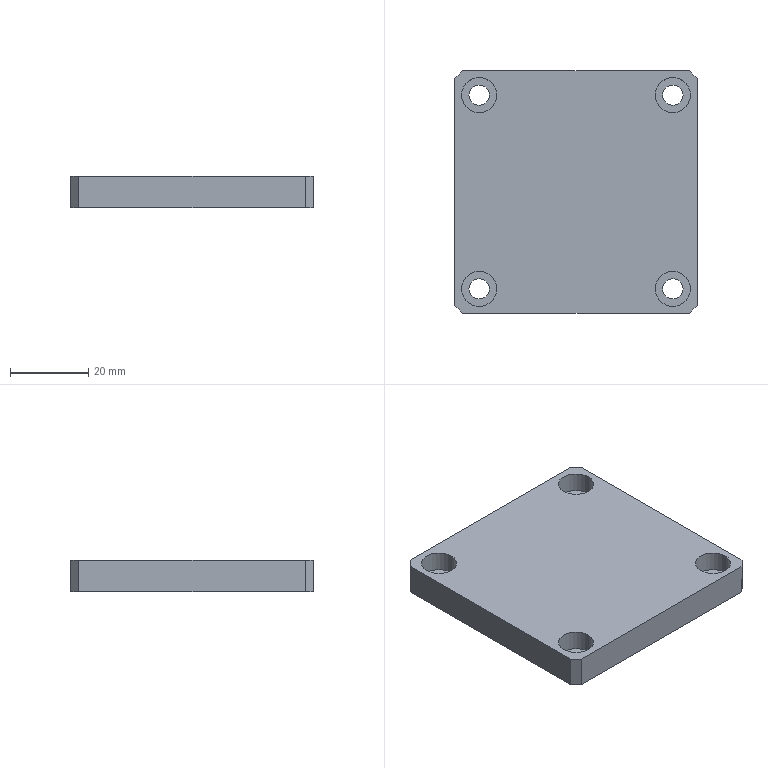Part | STEP file | 复件 FHB175-034^FHB175S-PRW-P40(马达RightUpper折-400W伺服电机) | 1 solid | 30 faces | box 62 x 62 x 8 mm | volume 29127 mm3 | cylinder 16 | plane 14 | commonest cylinder face diameters 5.2 x8 9 x8
STEP:
#1=CARTESIAN_POINT('',(-100.156,-108.498,0.));
#2=VERTEX_POINT('',#1);
#3=CARTESIAN_POINT('',(-105.356,-108.498,0.));
#4=VERTEX_POINT('',#3);
#5=CARTESIAN_POINT('',(-102.756,-108.498,0.));
#6=DIRECTION('',(0.,0.,-1.));
#7=DIRECTION('',(1.,0.,0.));
#8=AXIS2_PLACEMENT_3D('',#5,#6,#7);
#9=CIRCLE('',#8,2.6);
#10=EDGE_CURVE('',#2,#4,#9,.T.);
#11=ORIENTED_EDGE('',*,*,#10,.T.);
#12=CARTESIAN_POINT('',(-105.356,-108.498,2.8));
#13=VERTEX_POINT('',#12);
#14=CARTESIAN_POINT('',(-105.356,-108.498,8.));
#15=DIRECTION('',(0.,0.,1.));
#16=VECTOR('',#15,1000.);
#17=LINE('',#14,#16);
#18=EDGE_CURVE('',#4,#13,#17,.T.);
#19=ORIENTED_EDGE('',*,*,#18,.T.);
#20=CARTESIAN_POINT('',(-100.156,-108.498,2.8));
#21=VERTEX_POINT('',#20);
#22=CARTESIAN_POINT('',(-102.756,-108.498,2.8));
#23=DIRECTION('',(0.,0.,-1.));
#24=DIRECTION('',(1.,0.,0.));
#25=AXIS2_PLACEMENT_3D('',#22,#23,#24);
#26=CIRCLE('',#25,2.6);
#27=EDGE_CURVE('',#21,#13,#26,.T.);
#28=ORIENTED_EDGE('',*,*,#27,.F.);
#29=CARTESIAN_POINT('',(-100.156,-108.498,8.));
#30=DIRECTION('',(0.,0.,1.));
#31=VECTOR('',#30,1000.);
#32=LINE('',#29,#31);
#33=EDGE_CURVE('',#2,#21,#32,.T.);
#34=ORIENTED_EDGE('',*,*,#33,.F.);
#35=EDGE_LOOP('',(#11,#19,#28,#34));
#36=FACE_OUTER_BOUND('',#35,.T.);
#37=CARTESIAN_POINT('',(-102.756,-108.498,8.));
#38=DIRECTION('',(0.,0.,1.));
#39=DIRECTION('',(1.,0.,0.));
#40=AXIS2_PLACEMENT_3D('',#37,#38,#39);
#41=CYLINDRICAL_SURFACE('',#40,2.6);
#42=ADVANCED_FACE('',(#36),#41,.F.);
#43=CARTESIAN_POINT('',(-50.656,-108.498,0.));
#44=VERTEX_POINT('',#43);
#45=CARTESIAN_POINT('',(-55.856,-108.498,0.));
#46=VERTEX_POINT('',#45);
#47=CARTESIAN_POINT('',(-53.256,-108.498,0.));
#48=DIRECTION('',(0.,0.,-1.));
#49=DIRECTION('',(1.,0.,0.));
#50=AXIS2_PLACEMENT_3D('',#47,#48,#49);
#51=CIRCLE('',#50,2.6);
#52=EDGE_CURVE('',#44,#46,#51,.T.);
#53=ORIENTED_EDGE('',*,*,#52,.T.);
#54=CARTESIAN_POINT('',(-55.856,-108.498,2.8));
#55=VERTEX_POINT('',#54);
#56=CARTESIAN_POINT('',(-55.856,-108.498,8.));
#57=DIRECTION('',(0.,0.,1.));
#58=VECTOR('',#57,1000.);
#59=LINE('',#56,#58);
#60=EDGE_CURVE('',#46,#55,#59,.T.);
#61=ORIENTED_EDGE('',*,*,#60,.T.);
#62=CARTESIAN_POINT('',(-50.656,-108.498,2.8));
#63=VERTEX_POINT('',#62);
#64=CARTESIAN_POINT('',(-53.256,-108.498,2.8));
#65=DIRECTION('',(0.,0.,-1.));
#66=DIRECTION('',(1.,0.,0.));
#67=AXIS2_PLACEMENT_3D('',#64,#65,#66);
#68=CIRCLE('',#67,2.6);
#69=EDGE_CURVE('',#63,#55,#68,.T.);
#70=ORIENTED_EDGE('',*,*,#69,.F.);
#71=CARTESIAN_POINT('',(-50.656,-108.498,8.));
#72=DIRECTION('',(0.,0.,1.));
#73=VECTOR('',#72,1000.);
#74=LINE('',#71,#73);
#75=EDGE_CURVE('',#44,#63,#74,.T.);
#76=ORIENTED_EDGE('',*,*,#75,.F.);
#77=EDGE_LOOP('',(#53,#61,#70,#76));
#78=FACE_OUTER_BOUND('',#77,.T.);
#79=CARTESIAN_POINT('',(-53.256,-108.498,8.));
#80=DIRECTION('',(0.,0.,1.));
#81=DIRECTION('',(1.,0.,0.));
#82=AXIS2_PLACEMENT_3D('',#79,#80,#81);
#83=CYLINDRICAL_SURFACE('',#82,2.6);
#84=ADVANCED_FACE('',(#78),#83,.F.);
#85=CARTESIAN_POINT('',(-50.656,-58.998,0.));
#86=VERTEX_POINT('',#85);
#87=CARTESIAN_POINT('',(-55.856,-58.998,0.));
#88=VERTEX_POINT('',#87);
#89=CARTESIAN_POINT('',(-53.256,-58.998,0.));
#90=DIRECTION('',(0.,0.,-1.));
#91=DIRECTION('',(1.,0.,0.));
#92=AXIS2_PLACEMENT_3D('',#89,#90,#91);
#93=CIRCLE('',#92,2.6);
#94=EDGE_CURVE('',#86,#88,#93,.T.);
#95=ORIENTED_EDGE('',*,*,#94,.T.);
#96=CARTESIAN_POINT('',(-55.856,-58.998,2.8));
#97=VERTEX_POINT('',#96);
#98=CARTESIAN_POINT('',(-55.856,-58.998,8.));
#99=DIRECTION('',(0.,0.,1.));
#100=VECTOR('',#99,1000.);
#101=LINE('',#98,#100);
#102=EDGE_CURVE('',#88,#97,#101,.T.);
#103=ORIENTED_EDGE('',*,*,#102,.T.);
#104=CARTESIAN_POINT('',(-50.656,-58.998,2.8));
#105=VERTEX_POINT('',#104);
#106=CARTESIAN_POINT('',(-53.256,-58.998,2.8));
#107=DIRECTION('',(0.,0.,-1.));
#108=DIRECTION('',(1.,0.,0.));
#109=AXIS2_PLACEMENT_3D('',#106,#107,#108);
#110=CIRCLE('',#109,2.6);
#111=EDGE_CURVE('',#105,#97,#110,.T.);
#112=ORIENTED_EDGE('',*,*,#111,.F.);
#113=CARTESIAN_POINT('',(-50.656,-58.998,8.));
#114=DIRECTION('',(0.,0.,1.));
#115=VECTOR('',#114,1000.);
#116=LINE('',#113,#115);
#117=EDGE_CURVE('',#86,#105,#116,.T.);
#118=ORIENTED_EDGE('',*,*,#117,.F.);
#119=EDGE_LOOP('',(#95,#103,#112,#118));
#120=FACE_OUTER_BOUND('',#119,.T.);
#121=CARTESIAN_POINT('',(-53.256,-58.998,8.));
#122=DIRECTION('',(0.,0.,1.));
#123=DIRECTION('',(1.,0.,0.));
#124=AXIS2_PLACEMENT_3D('',#121,#122,#123);
#125=CYLINDRICAL_SURFACE('',#124,2.6);
#126=ADVANCED_FACE('',(#120),#125,.F.);
#127=CARTESIAN_POINT('',(-100.156,-58.998,0.));
#128=VERTEX_POINT('',#127);
#129=CARTESIAN_POINT('',(-105.356,-58.998,0.));
#130=VERTEX_POINT('',#129);
#131=CARTESIAN_POINT('',(-102.756,-58.998,0.));
#132=DIRECTION('',(0.,0.,-1.));
#133=DIRECTION('',(1.,0.,0.));
#134=AXIS2_PLACEMENT_3D('',#131,#132,#133);
#135=CIRCLE('',#134,2.6);
#136=EDGE_CURVE('',#128,#130,#135,.T.);
#137=ORIENTED_EDGE('',*,*,#136,.T.);
#138=CARTESIAN_POINT('',(-105.356,-58.998,2.8));
#139=VERTEX_POINT('',#138);
#140=CARTESIAN_POINT('',(-105.356,-58.998,8.));
#141=DIRECTION('',(0.,0.,1.));
#142=VECTOR('',#141,1000.);
#143=LINE('',#140,#142);
#144=EDGE_CURVE('',#130,#139,#143,.T.);
#145=ORIENTED_EDGE('',*,*,#144,.T.);
#146=CARTESIAN_POINT('',(-100.156,-58.998,2.8));
#147=VERTEX_POINT('',#146);
#148=CARTESIAN_POINT('',(-102.756,-58.998,2.8));
#149=DIRECTION('',(0.,0.,-1.));
#150=DIRECTION('',(1.,0.,0.));
#151=AXIS2_PLACEMENT_3D('',#148,#149,#150);
#152=CIRCLE('',#151,2.6);
#153=EDGE_CURVE('',#147,#139,#152,.T.);
#154=ORIENTED_EDGE('',*,*,#153,.F.);
#155=CARTESIAN_POINT('',(-100.156,-58.998,8.));
#156=DIRECTION('',(0.,0.,1.));
#157=VECTOR('',#156,1000.);
#158=LINE('',#155,#157);
#159=EDGE_CURVE('',#128,#147,#158,.T.);
#160=ORIENTED_EDGE('',*,*,#159,.F.);
#161=EDGE_LOOP('',(#137,#145,#154,#160));
#162=FACE_OUTER_BOUND('',#161,.T.);
#163=CARTESIAN_POINT('',(-102.756,-58.998,8.));
#164=DIRECTION('',(0.,0.,1.));
#165=DIRECTION('',(1.,0.,0.));
#166=AXIS2_PLACEMENT_3D('',#163,#164,#165);
#167=CYLINDRICAL_SURFACE('',#166,2.6);
#168=ADVANCED_FACE('',(#162),#167,.F.);
#169=CARTESIAN_POINT('',(-98.256,-108.498,2.8));
#170=VERTEX_POINT('',#169);
#171=CARTESIAN_POINT('',(-107.256,-108.498,2.8));
#172=VERTEX_POINT('',#171);
#173=CARTESIAN_POINT('',(-102.756,-108.498,2.8));
#174=DIRECTION('',(0.,0.,-1.));
#175=DIRECTION('',(1.,0.,0.));
#176=AXIS2_PLACEMENT_3D('',#173,#174,#175);
#177=CIRCLE('',#176,4.5);
#178=EDGE_CURVE('',#170,#172,#177,.T.);
#179=ORIENTED_EDGE('',*,*,#178,.T.);
#180=CARTESIAN_POINT('',(-107.256,-108.498,8.));
#181=VERTEX_POINT('',#180);
#182=CARTESIAN_POINT('',(-107.256,-108.498,8.));
#183=DIRECTION('',(0.,0.,1.));
#184=VECTOR('',#183,1000.);
#185=LINE('',#182,#184);
#186=EDGE_CURVE('',#172,#181,#185,.T.);
#187=ORIENTED_EDGE('',*,*,#186,.T.);
#188=CARTESIAN_POINT('',(-98.256,-108.498,8.));
#189=VERTEX_POINT('',#188);
#190=CARTESIAN_POINT('',(-102.756,-108.498,8.));
#191=DIRECTION('',(0.,0.,-1.));
#192=DIRECTION('',(1.,0.,0.));
#193=AXIS2_PLACEMENT_3D('',#190,#191,#192);
#194=CIRCLE('',#193,4.5);
#195=EDGE_CURVE('',#189,#181,#194,.T.);
#196=ORIENTED_EDGE('',*,*,#195,.F.);
#197=CARTESIAN_POINT('',(-98.256,-108.498,8.));
#198=DIRECTION('',(0.,0.,1.));
#199=VECTOR('',#198,1000.);
#200=LINE('',#197,#199);
#201=EDGE_CURVE('',#170,#189,#200,.T.);
#202=ORIENTED_EDGE('',*,*,#201,.F.);
#203=EDGE_LOOP('',(#179,#187,#196,#202));
#204=FACE_OUTER_BOUND('',#203,.T.);
#205=CARTESIAN_POINT('',(-102.756,-108.498,8.));
#206=DIRECTION('',(0.,0.,1.));
#207=DIRECTION('',(1.,0.,0.));
#208=AXIS2_PLACEMENT_3D('',#205,#206,#207);
#209=CYLINDRICAL_SURFACE('',#208,4.5);
#210=ADVANCED_FACE('',(#204),#209,.F.);
#211=CARTESIAN_POINT('',(-48.756,-108.498,2.8));
#212=VERTEX_POINT('',#211);
#213=CARTESIAN_POINT('',(-57.756,-108.498,2.8));
#214=VERTEX_POINT('',#213);
#215=CARTESIAN_POINT('',(-53.256,-108.498,2.8));
#216=DIRECTION('',(0.,0.,-1.));
#217=DIRECTION('',(1.,0.,0.));
#218=AXIS2_PLACEMENT_3D('',#215,#216,#217);
#219=CIRCLE('',#218,4.5);
#220=EDGE_CURVE('',#212,#214,#219,.T.);
#221=ORIENTED_EDGE('',*,*,#220,.T.);
#222=CARTESIAN_POINT('',(-57.756,-108.498,8.));
#223=VERTEX_POINT('',#222);
#224=CARTESIAN_POINT('',(-57.756,-108.498,8.));
#225=DIRECTION('',(0.,0.,1.));
#226=VECTOR('',#225,1000.);
#227=LINE('',#224,#226);
#228=EDGE_CURVE('',#214,#223,#227,.T.);
#229=ORIENTED_EDGE('',*,*,#228,.T.);
#230=CARTESIAN_POINT('',(-48.756,-108.498,8.));
#231=VERTEX_POINT('',#230);
#232=CARTESIAN_POINT('',(-53.256,-108.498,8.));
#233=DIRECTION('',(0.,0.,-1.));
#234=DIRECTION('',(1.,0.,0.));
#235=AXIS2_PLACEMENT_3D('',#232,#233,#234);
#236=CIRCLE('',#235,4.5);
#237=EDGE_CURVE('',#231,#223,#236,.T.);
#238=ORIENTED_EDGE('',*,*,#237,.F.);
#239=CARTESIAN_POINT('',(-48.756,-108.498,8.));
#240=DIRECTION('',(0.,0.,1.));
#241=VECTOR('',#240,1000.);
#242=LINE('',#239,#241);
#243=EDGE_CURVE('',#212,#231,#242,.T.);
#244=ORIENTED_EDGE('',*,*,#243,.F.);
#245=EDGE_LOOP('',(#221,#229,#238,#244));
#246=FACE_OUTER_BOUND('',#245,.T.);
#247=CARTESIAN_POINT('',(-53.256,-108.498,8.));
#248=DIRECTION('',(0.,0.,1.));
#249=DIRECTION('',(1.,0.,0.));
#250=AXIS2_PLACEMENT_3D('',#247,#248,#249);
#251=CYLINDRICAL_SURFACE('',#250,4.5);
#252=ADVANCED_FACE('',(#246),#251,.F.);
#253=CARTESIAN_POINT('',(-48.756,-58.998,2.8));
#254=VERTEX_POINT('',#253);
#255=CARTESIAN_POINT('',(-57.756,-58.998,2.8));
#256=VERTEX_POINT('',#255);
#257=CARTESIAN_POINT('',(-53.256,-58.998,2.8));
#258=DIRECTION('',(0.,0.,-1.));
#259=DIRECTION('',(1.,0.,0.));
#260=AXIS2_PLACEMENT_3D('',#257,#258,#259);
#261=CIRCLE('',#260,4.5);
#262=EDGE_CURVE('',#254,#256,#261,.T.);
#263=ORIENTED_EDGE('',*,*,#262,.T.);
#264=CARTESIAN_POINT('',(-57.756,-58.998,8.));
#265=VERTEX_POINT('',#264);
#266=CARTESIAN_POINT('',(-57.756,-58.998,8.));
#267=DIRECTION('',(0.,0.,1.));
#268=VECTOR('',#267,1000.);
#269=LINE('',#266,#268);
#270=EDGE_CURVE('',#256,#265,#269,.T.);
#271=ORIENTED_EDGE('',*,*,#270,.T.);
#272=CARTESIAN_POINT('',(-48.756,-58.998,8.));
#273=VERTEX_POINT('',#272);
#274=CARTESIAN_POINT('',(-53.256,-58.998,8.));
#275=DIRECTION('',(0.,0.,-1.));
#276=DIRECTION('',(1.,0.,0.));
#277=AXIS2_PLACEMENT_3D('',#274,#275,#276);
#278=CIRCLE('',#277,4.5);
#279=EDGE_CURVE('',#273,#265,#278,.T.);
#280=ORIENTED_EDGE('',*,*,#279,.F.);
#281=CARTESIAN_POINT('',(-48.756,-58.998,8.));
#282=DIRECTION('',(0.,0.,1.));
#283=VECTOR('',#282,1000.);
#284=LINE('',#281,#283);
#285=EDGE_CURVE('',#254,#273,#284,.T.);
#286=ORIENTED_EDGE('',*,*,#285,.F.);
#287=EDGE_LOOP('',(#263,#271,#280,#286));
#288=FACE_OUTER_BOUND('',#287,.T.);
#289=CARTESIAN_POINT('',(-53.256,-58.998,8.));
#290=DIRECTION('',(0.,0.,1.));
#291=DIRECTION('',(1.,0.,0.));
#292=AXIS2_PLACEMENT_3D('',#289,#290,#291);
#293=CYLINDRICAL_SURFACE('',#292,4.5);
#294=ADVANCED_FACE('',(#288),#293,.F.);
#295=CARTESIAN_POINT('',(-98.256,-58.998,2.8));
#296=VERTEX_POINT('',#295);
#297=CARTESIAN_POINT('',(-107.256,-58.998,2.8));
#298=VERTEX_POINT('',#297);
#299=CARTESIAN_POINT('',(-102.756,-58.998,2.8));
#300=DIRECTION('',(0.,0.,-1.));
#301=DIRECTION('',(1.,0.,0.));
#302=AXIS2_PLACEMENT_3D('',#299,#300,#301);
#303=CIRCLE('',#302,4.5);
#304=EDGE_CURVE('',#296,#298,#303,.T.);
#305=ORIENTED_EDGE('',*,*,#304,.T.);
#306=CARTESIAN_POINT('',(-107.256,-58.998,8.));
#307=VERTEX_POINT('',#306);
#308=CARTESIAN_POINT('',(-107.256,-58.998,8.));
#309=DIRECTION('',(0.,0.,1.));
#310=VECTOR('',#309,1000.);
#311=LINE('',#308,#310);
#312=EDGE_CURVE('',#298,#307,#311,.T.);
#313=ORIENTED_EDGE('',*,*,#312,.T.);
#314=CARTESIAN_POINT('',(-98.256,-58.998,8.));
#315=VERTEX_POINT('',#314);
#316=CARTESIAN_POINT('',(-102.756,-58.998,8.));
#317=DIRECTION('',(0.,0.,-1.));
#318=DIRECTION('',(1.,0.,0.));
#319=AXIS2_PLACEMENT_3D('',#316,#317,#318);
#320=CIRCLE('',#319,4.5);
#321=EDGE_CURVE('',#315,#307,#320,.T.);
#322=ORIENTED_EDGE('',*,*,#321,.F.);
#323=CARTESIAN_POINT('',(-98.256,-58.998,8.));
#324=DIRECTION('',(0.,0.,1.));
#325=VECTOR('',#324,1000.);
#326=LINE('',#323,#325);
#327=EDGE_CURVE('',#296,#315,#326,.T.);
#328=ORIENTED_EDGE('',*,*,#327,.F.);
#329=EDGE_LOOP('',(#305,#313,#322,#328));
#330=FACE_OUTER_BOUND('',#329,.T.);
#331=CARTESIAN_POINT('',(-102.756,-58.998,8.));
#332=DIRECTION('',(0.,0.,1.));
#333=DIRECTION('',(1.,0.,0.));
#334=AXIS2_PLACEMENT_3D('',#331,#332,#333);
#335=CYLINDRICAL_SURFACE('',#334,4.5);
#336=ADVANCED_FACE('',(#330),#335,.F.);
#337=CARTESIAN_POINT('',(-109.006,-112.748,0.));
#338=VERTEX_POINT('',#337);
#339=CARTESIAN_POINT('',(-107.006,-114.748,0.));
#340=VERTEX_POINT('',#339);
#341=CARTESIAN_POINT('',(-109.006,-112.748,0.));
#342=DIRECTION('',(0.7071,-0.7071,0.));
#343=VECTOR('',#342,1000.);
#344=LINE('',#341,#343);
#345=EDGE_CURVE('',#338,#340,#344,.T.);
#346=ORIENTED_EDGE('',*,*,#345,.F.);
#347=CARTESIAN_POINT('',(-109.006,-54.748,0.));
#348=VERTEX_POINT('',#347);
#349=CARTESIAN_POINT('',(-109.006,0.,0.));
#350=DIRECTION('',(0.,-1.,0.));
#351=VECTOR('',#350,1000.);
#352=LINE('',#349,#351);
#353=EDGE_CURVE('',#348,#338,#352,.T.);
#354=ORIENTED_EDGE('',*,*,#353,.F.);
#355=CARTESIAN_POINT('',(-107.006,-52.748,0.));
#356=VERTEX_POINT('',#355);
#357=CARTESIAN_POINT('',(-107.006,-52.748,0.));
#358=DIRECTION('',(-0.7071,-0.7071,0.));
#359=VECTOR('',#358,1000.);
#360=LINE('',#357,#359);
#361=EDGE_CURVE('',#356,#348,#360,.T.);
#362=ORIENTED_EDGE('',*,*,#361,.F.);
#363=CARTESIAN_POINT('',(-49.006,-52.748,0.));
#364=VERTEX_POINT('',#363);
#365=CARTESIAN_POINT('',(0.,-52.748,0.));
#366=DIRECTION('',(-1.,0.,0.));
#367=VECTOR('',#366,1000.);
#368=LINE('',#365,#367);
#369=EDGE_CURVE('',#364,#356,#368,.T.);
#370=ORIENTED_EDGE('',*,*,#369,.F.);
#371=CARTESIAN_POINT('',(-47.006,-54.748,0.));
#372=VERTEX_POINT('',#371);
#373=CARTESIAN_POINT('',(-47.006,-54.748,0.));
#374=DIRECTION('',(-0.7071,0.7071,0.));
#375=VECTOR('',#374,1000.);
#376=LINE('',#373,#375);
#377=EDGE_CURVE('',#372,#364,#376,.T.);
#378=ORIENTED_EDGE('',*,*,#377,.F.);
#379=CARTESIAN_POINT('',(-47.006,-112.748,0.));
#380=VERTEX_POINT('',#379);
#381=CARTESIAN_POINT('',(-47.006,0.,0.));
#382=DIRECTION('',(0.,1.,0.));
#383=VECTOR('',#382,1000.);
#384=LINE('',#381,#383);
#385=EDGE_CURVE('',#380,#372,#384,.T.);
#386=ORIENTED_EDGE('',*,*,#385,.F.);
#387=CARTESIAN_POINT('',(-49.006,-114.748,0.));
#388=VERTEX_POINT('',#387);
#389=CARTESIAN_POINT('',(-49.006,-114.748,0.));
#390=DIRECTION('',(0.7071,0.7071,0.));
#391=VECTOR('',#390,1000.);
#392=LINE('',#389,#391);
#393=EDGE_CURVE('',#388,#380,#392,.T.);
#394=ORIENTED_EDGE('',*,*,#393,.F.);
#395=CARTESIAN_POINT('',(0.,-114.748,0.));
#396=DIRECTION('',(1.,0.,0.));
#397=VECTOR('',#396,1000.);
#398=LINE('',#395,#397);
#399=EDGE_CURVE('',#340,#388,#398,.T.);
#400=ORIENTED_EDGE('',*,*,#399,.F.);
#401=EDGE_LOOP('',(#346,#354,#362,#370,#378,#386,#394,#400));
#402=FACE_OUTER_BOUND('',#401,.T.);
#403=ORIENTED_EDGE('',*,*,#10,.F.);
#404=CARTESIAN_POINT('',(-102.756,-108.498,0.));
#405=DIRECTION('',(0.,0.,-1.));
#406=DIRECTION('',(1.,0.,0.));
#407=AXIS2_PLACEMENT_3D('',#404,#405,#406);
#408=CIRCLE('',#407,2.6);
#409=EDGE_CURVE('',#4,#2,#408,.T.);
#410=ORIENTED_EDGE('',*,*,#409,.F.);
#411=EDGE_LOOP('',(#403,#410));
#412=FACE_BOUND('',#411,.T.);
#413=ORIENTED_EDGE('',*,*,#52,.F.);
#414=CARTESIAN_POINT('',(-53.256,-108.498,0.));
#415=DIRECTION('',(0.,0.,-1.));
#416=DIRECTION('',(1.,0.,0.));
#417=AXIS2_PLACEMENT_3D('',#414,#415,#416);
#418=CIRCLE('',#417,2.6);
#419=EDGE_CURVE('',#46,#44,#418,.T.);
#420=ORIENTED_EDGE('',*,*,#419,.F.);
#421=EDGE_LOOP('',(#413,#420));
#422=FACE_BOUND('',#421,.T.);
#423=ORIENTED_EDGE('',*,*,#94,.F.);
#424=CARTESIAN_POINT('',(-53.256,-58.998,0.));
#425=DIRECTION('',(0.,0.,-1.));
#426=DIRECTION('',(1.,0.,0.));
#427=AXIS2_PLACEMENT_3D('',#424,#425,#426);
#428=CIRCLE('',#427,2.6);
#429=EDGE_CURVE('',#88,#86,#428,.T.);
#430=ORIENTED_EDGE('',*,*,#429,.F.);
#431=EDGE_LOOP('',(#423,#430));
#432=FACE_BOUND('',#431,.T.);
#433=ORIENTED_EDGE('',*,*,#136,.F.);
#434=CARTESIAN_POINT('',(-102.756,-58.998,0.));
#435=DIRECTION('',(0.,0.,-1.));
#436=DIRECTION('',(1.,0.,0.));
#437=AXIS2_PLACEMENT_3D('',#434,#435,#436);
#438=CIRCLE('',#437,2.6);
#439=EDGE_CURVE('',#130,#128,#438,.T.);
#440=ORIENTED_EDGE('',*,*,#439,.F.);
#441=EDGE_LOOP('',(#433,#440));
#442=FACE_BOUND('',#441,.T.);
#443=CARTESIAN_POINT('',(0.,0.,0.));
#444=DIRECTION('',(0.,0.,1.));
#445=DIRECTION('',(1.,0.,0.));
#446=AXIS2_PLACEMENT_3D('',#443,#444,#445);
#447=PLANE('',#446);
#448=ADVANCED_FACE('',(#402,#412,#422,#432,#442),#447,.F.);
#449=CARTESIAN_POINT('',(-107.006,-114.748,8.));
#450=VERTEX_POINT('',#449);
#451=CARTESIAN_POINT('',(-107.006,-114.748,8.));
#452=DIRECTION('',(0.,0.,1.));
#453=VECTOR('',#452,1000.);
#454=LINE('',#451,#453);
#455=EDGE_CURVE('',#340,#450,#454,.T.);
#456=ORIENTED_EDGE('',*,*,#455,.F.);
#457=ORIENTED_EDGE('',*,*,#399,.T.);
#458=CARTESIAN_POINT('',(-49.006,-114.748,8.));
#459=VERTEX_POINT('',#458);
#460=CARTESIAN_POINT('',(-49.006,-114.748,8.));
#461=DIRECTION('',(0.,0.,-1.));
#462=VECTOR('',#461,1000.);
#463=LINE('',#460,#462);
#464=EDGE_CURVE('',#459,#388,#463,.T.);
#465=ORIENTED_EDGE('',*,*,#464,.F.);
#466=CARTESIAN_POINT('',(-109.006,-114.748,8.));
#467=DIRECTION('',(1.,0.,0.));
#468=VECTOR('',#467,1000.);
#469=LINE('',#466,#468);
#470=EDGE_CURVE('',#450,#459,#469,.T.);
#471=ORIENTED_EDGE('',*,*,#470,.F.);
#472=EDGE_LOOP('',(#456,#457,#465,#471));
#473=FACE_OUTER_BOUND('',#472,.T.);
#474=CARTESIAN_POINT('',(-109.006,-114.748,8.));
#475=DIRECTION('',(0.,1.,0.));
#476=DIRECTION('',(0.,0.,1.));
#477=AXIS2_PLACEMENT_3D('',#474,#475,#476);
#478=PLANE('',#477);
#479=ADVANCED_FACE('',(#473),#478,.F.);
#480=CARTESIAN_POINT('',(-109.006,-112.748,8.));
#481=VERTEX_POINT('',#480);
#482=CARTESIAN_POINT('',(-109.006,-112.748,8.));
#483=DIRECTION('',(0.,0.,1.));
#484=VECTOR('',#483,1000.);
#485=LINE('',#482,#484);
#486=EDGE_CURVE('',#338,#481,#485,.T.);
#487=ORIENTED_EDGE('',*,*,#486,.F.);
#488=ORIENTED_EDGE('',*,*,#345,.T.);
#489=ORIENTED_EDGE('',*,*,#455,.T.);
#490=CARTESIAN_POINT('',(-107.006,-114.748,8.));
#491=DIRECTION('',(0.7071,-0.7071,0.));
#492=VECTOR('',#491,1000.);
#493=LINE('',#490,#492);
#494=EDGE_CURVE('',#481,#450,#493,.T.);
#495=ORIENTED_EDGE('',*,*,#494,.F.);
#496=EDGE_LOOP('',(#487,#488,#489,#495));
#497=FACE_OUTER_BOUND('',#496,.T.);
#498=CARTESIAN_POINT('',(-107.006,-114.748,8.));
#499=DIRECTION('',(0.7071,0.7071,0.));
#500=DIRECTION('',(-0.7071,0.7071,0.));
#501=AXIS2_PLACEMENT_3D('',#498,#499,#500);
#502=PLANE('',#501);
#503=ADVANCED_FACE('',(#497),#502,.F.);
#504=ORIENTED_EDGE('',*,*,#486,.T.);
#505=CARTESIAN_POINT('',(-109.006,-54.748,8.));
#506=VERTEX_POINT('',#505);
#507=CARTESIAN_POINT('',(-109.006,-52.748,8.));
#508=DIRECTION('',(0.,-1.,0.));
#509=VECTOR('',#508,1000.);
#510=LINE('',#507,#509);
#511=EDGE_CURVE('',#506,#481,#510,.T.);
#512=ORIENTED_EDGE('',*,*,#511,.F.);
#513=CARTESIAN_POINT('',(-109.006,-54.748,8.));
#514=DIRECTION('',(0.,0.,1.));
#515=VECTOR('',#514,1000.);
#516=LINE('',#513,#515);
#517=EDGE_CURVE('',#348,#506,#516,.T.);
#518=ORIENTED_EDGE('',*,*,#517,.F.);
#519=ORIENTED_EDGE('',*,*,#353,.T.);
#520=EDGE_LOOP('',(#504,#512,#518,#519));
#521=FACE_OUTER_BOUND('',#520,.T.);
#522=CARTESIAN_POINT('',(-109.006,-52.748,8.));
#523=DIRECTION('',(1.,0.,0.));
#524=DIRECTION('',(0.,0.,-1.));
#525=AXIS2_PLACEMENT_3D('',#522,#523,#524);
#526=PLANE('',#525);
#527=ADVANCED_FACE('',(#521),#526,.F.);
#528=CARTESIAN_POINT('',(-107.006,-52.748,8.));
#529=VERTEX_POINT('',#528);
#530=CARTESIAN_POINT('',(-107.006,-52.748,8.));
#531=DIRECTION('',(0.,0.,1.));
#532=VECTOR('',#531,1000.);
#533=LINE('',#530,#532);
#534=EDGE_CURVE('',#356,#529,#533,.T.);
#535=ORIENTED_EDGE('',*,*,#534,.F.);
#536=ORIENTED_EDGE('',*,*,#361,.T.);
#537=ORIENTED_EDGE('',*,*,#517,.T.);
#538=CARTESIAN_POINT('',(-109.006,-54.748,8.));
#539=DIRECTION('',(-0.7071,-0.7071,0.));
#540=VECTOR('',#539,1000.);
#541=LINE('',#538,#540);
#542=EDGE_CURVE('',#529,#506,#541,.T.);
#543=ORIENTED_EDGE('',*,*,#542,.F.);
#544=EDGE_LOOP('',(#535,#536,#537,#543));
#545=FACE_OUTER_BOUND('',#544,.T.);
#546=CARTESIAN_POINT('',(-109.006,-54.748,8.));
#547=DIRECTION('',(0.7071,-0.7071,0.));
#548=DIRECTION('',(0.7071,0.7071,0.));
#549=AXIS2_PLACEMENT_3D('',#546,#547,#548);
#550=PLANE('',#549);
#551=ADVANCED_FACE('',(#545),#550,.F.);
#552=CARTESIAN_POINT('',(-49.006,-52.748,8.));
#553=VERTEX_POINT('',#552);
#554=CARTESIAN_POINT('',(-49.006,-52.748,8.));
#555=DIRECTION('',(0.,0.,1.));
#556=VECTOR('',#555,1000.);
#557=LINE('',#554,#556);
#558=EDGE_CURVE('',#364,#553,#557,.T.);
#559=ORIENTED_EDGE('',*,*,#558,.F.);
#560=ORIENTED_EDGE('',*,*,#369,.T.);
#561=ORIENTED_EDGE('',*,*,#534,.T.);
#562=CARTESIAN_POINT('',(-109.006,-52.748,8.));
#563=DIRECTION('',(-1.,0.,0.));
#564=VECTOR('',#563,1000.);
#565=LINE('',#562,#564);
#566=EDGE_CURVE('',#553,#529,#565,.T.);
#567=ORIENTED_EDGE('',*,*,#566,.F.);
#568=EDGE_LOOP('',(#559,#560,#561,#567));
#569=FACE_OUTER_BOUND('',#568,.T.);
#570=CARTESIAN_POINT('',(-109.006,-52.748,8.));
#571=DIRECTION('',(0.,-1.,0.));
#572=DIRECTION('',(0.,0.,-1.));
#573=AXIS2_PLACEMENT_3D('',#570,#571,#572);
#574=PLANE('',#573);
#575=ADVANCED_FACE('',(#569),#574,.F.);
#576=CARTESIAN_POINT('',(-47.006,-54.748,8.));
#577=VERTEX_POINT('',#576);
#578=CARTESIAN_POINT('',(-47.006,-54.748,8.));
#579=DIRECTION('',(0.,0.,1.));
#580=VECTOR('',#579,1000.);
#581=LINE('',#578,#580);
#582=EDGE_CURVE('',#372,#577,#581,.T.);
#583=ORIENTED_EDGE('',*,*,#582,.F.);
#584=ORIENTED_EDGE('',*,*,#377,.T.);
#585=ORIENTED_EDGE('',*,*,#558,.T.);
#586=CARTESIAN_POINT('',(-49.006,-52.748,8.));
#587=DIRECTION('',(-0.7071,0.7071,0.));
#588=VECTOR('',#587,1000.);
#589=LINE('',#586,#588);
#590=EDGE_CURVE('',#577,#553,#589,.T.);
#591=ORIENTED_EDGE('',*,*,#590,.F.);
#592=EDGE_LOOP('',(#583,#584,#585,#591));
#593=FACE_OUTER_BOUND('',#592,.T.);
#594=CARTESIAN_POINT('',(-49.006,-52.748,8.));
#595=DIRECTION('',(-0.7071,-0.7071,0.));
#596=DIRECTION('',(0.7071,-0.7071,0.));
#597=AXIS2_PLACEMENT_3D('',#594,#595,#596);
#598=PLANE('',#597);
#599=ADVANCED_FACE('',(#593),#598,.F.);
#600=CARTESIAN_POINT('',(-47.006,-112.748,8.));
#601=VERTEX_POINT('',#600);
#602=CARTESIAN_POINT('',(-47.006,-112.748,8.));
#603=DIRECTION('',(0.,0.,1.));
#604=VECTOR('',#603,1000.);
#605=LINE('',#602,#604);
#606=EDGE_CURVE('',#380,#601,#605,.T.);
#607=ORIENTED_EDGE('',*,*,#606,.F.);
#608=ORIENTED_EDGE('',*,*,#385,.T.);
#609=ORIENTED_EDGE('',*,*,#582,.T.);
#610=CARTESIAN_POINT('',(-47.006,-52.748,8.));
#611=DIRECTION('',(0.,1.,0.));
#612=VECTOR('',#611,1000.);
#613=LINE('',#610,#612);
#614=EDGE_CURVE('',#601,#577,#613,.T.);
#615=ORIENTED_EDGE('',*,*,#614,.F.);
#616=EDGE_LOOP('',(#607,#608,#609,#615));
#617=FACE_OUTER_BOUND('',#616,.T.);
#618=CARTESIAN_POINT('',(-47.006,-52.748,8.));
#619=DIRECTION('',(-1.,0.,0.));
#620=DIRECTION('',(0.,-1.,0.));
#621=AXIS2_PLACEMENT_3D('',#618,#619,#620);
#622=PLANE('',#621);
#623=ADVANCED_FACE('',(#617),#622,.F.);
#624=ORIENTED_EDGE('',*,*,#464,.T.);
#625=ORIENTED_EDGE('',*,*,#393,.T.);
#626=ORIENTED_EDGE('',*,*,#606,.T.);
#627=CARTESIAN_POINT('',(-47.006,-112.748,8.));
#628=DIRECTION('',(0.7071,0.7071,0.));
#629=VECTOR('',#628,1000.);
#630=LINE('',#627,#629);
#631=EDGE_CURVE('',#459,#601,#630,.T.);
#632=ORIENTED_EDGE('',*,*,#631,.F.);
#633=EDGE_LOOP('',(#624,#625,#626,#632));
#634=FACE_OUTER_BOUND('',#633,.T.);
#635=CARTESIAN_POINT('',(-47.006,-112.748,8.));
#636=DIRECTION('',(-0.7071,0.7071,0.));
#637=DIRECTION('',(-0.7071,-0.7071,0.));
#638=AXIS2_PLACEMENT_3D('',#635,#636,#637);
#639=PLANE('',#638);
#640=ADVANCED_FACE('',(#634),#639,.F.);
#641=ORIENTED_EDGE('',*,*,#18,.F.);
#642=ORIENTED_EDGE('',*,*,#409,.T.);
#643=ORIENTED_EDGE('',*,*,#33,.T.);
#644=CARTESIAN_POINT('',(-102.756,-108.498,2.8));
#645=DIRECTION('',(0.,0.,-1.));
#646=DIRECTION('',(1.,0.,0.));
#647=AXIS2_PLACEMENT_3D('',#644,#645,#646);
#648=CIRCLE('',#647,2.6);
#649=EDGE_CURVE('',#13,#21,#648,.T.);
#650=ORIENTED_EDGE('',*,*,#649,.F.);
#651=EDGE_LOOP('',(#641,#642,#643,#650));
#652=FACE_OUTER_BOUND('',#651,.T.);
#653=CARTESIAN_POINT('',(-102.756,-108.498,8.));
#654=DIRECTION('',(0.,0.,1.));
#655=DIRECTION('',(1.,0.,0.));
#656=AXIS2_PLACEMENT_3D('',#653,#654,#655);
#657=CYLINDRICAL_SURFACE('',#656,2.6);
#658=ADVANCED_FACE('',(#652),#657,.F.);
#659=ORIENTED_EDGE('',*,*,#60,.F.);
#660=ORIENTED_EDGE('',*,*,#419,.T.);
#661=ORIENTED_EDGE('',*,*,#75,.T.);
#662=CARTESIAN_POINT('',(-53.256,-108.498,2.8));
#663=DIRECTION('',(0.,0.,-1.));
#664=DIRECTION('',(1.,0.,0.));
#665=AXIS2_PLACEMENT_3D('',#662,#663,#664);
#666=CIRCLE('',#665,2.6);
#667=EDGE_CURVE('',#55,#63,#666,.T.);
#668=ORIENTED_EDGE('',*,*,#667,.F.);
#669=EDGE_LOOP('',(#659,#660,#661,#668));
#670=FACE_OUTER_BOUND('',#669,.T.);
#671=CARTESIAN_POINT('',(-53.256,-108.498,8.));
#672=DIRECTION('',(0.,0.,1.));
#673=DIRECTION('',(1.,0.,0.));
#674=AXIS2_PLACEMENT_3D('',#671,#672,#673);
#675=CYLINDRICAL_SURFACE('',#674,2.6);
#676=ADVANCED_FACE('',(#670),#675,.F.);
#677=ORIENTED_EDGE('',*,*,#102,.F.);
#678=ORIENTED_EDGE('',*,*,#429,.T.);
#679=ORIENTED_EDGE('',*,*,#117,.T.);
#680=CARTESIAN_POINT('',(-53.256,-58.998,2.8));
#681=DIRECTION('',(0.,0.,-1.));
#682=DIRECTION('',(1.,0.,0.));
#683=AXIS2_PLACEMENT_3D('',#680,#681,#682);
#684=CIRCLE('',#683,2.6);
#685=EDGE_CURVE('',#97,#105,#684,.T.);
#686=ORIENTED_EDGE('',*,*,#685,.F.);
#687=EDGE_LOOP('',(#677,#678,#679,#686));
#688=FACE_OUTER_BOUND('',#687,.T.);
#689=CARTESIAN_POINT('',(-53.256,-58.998,8.));
#690=DIRECTION('',(0.,0.,1.));
#691=DIRECTION('',(1.,0.,0.));
#692=AXIS2_PLACEMENT_3D('',#689,#690,#691);
#693=CYLINDRICAL_SURFACE('',#692,2.6);
#694=ADVANCED_FACE('',(#688),#693,.F.);
#695=ORIENTED_EDGE('',*,*,#144,.F.);
#696=ORIENTED_EDGE('',*,*,#439,.T.);
#697=ORIENTED_EDGE('',*,*,#159,.T.);
#698=CARTESIAN_POINT('',(-102.756,-58.998,2.8));
#699=DIRECTION('',(0.,0.,-1.));
#700=DIRECTION('',(1.,0.,0.));
#701=AXIS2_PLACEMENT_3D('',#698,#699,#700);
#702=CIRCLE('',#701,2.6);
#703=EDGE_CURVE('',#139,#147,#702,.T.);
#704=ORIENTED_EDGE('',*,*,#703,.F.);
#705=EDGE_LOOP('',(#695,#696,#697,#704));
#706=FACE_OUTER_BOUND('',#705,.T.);
#707=CARTESIAN_POINT('',(-102.756,-58.998,8.));
#708=DIRECTION('',(0.,0.,1.));
#709=DIRECTION('',(1.,0.,0.));
#710=AXIS2_PLACEMENT_3D('',#707,#708,#709);
#711=CYLINDRICAL_SURFACE('',#710,2.6);
#712=ADVANCED_FACE('',(#706),#711,.F.);
#713=ORIENTED_EDGE('',*,*,#566,.T.);
#714=ORIENTED_EDGE('',*,*,#542,.T.);
#715=ORIENTED_EDGE('',*,*,#511,.T.);
#716=ORIENTED_EDGE('',*,*,#494,.T.);
#717=ORIENTED_EDGE('',*,*,#470,.T.);
#718=ORIENTED_EDGE('',*,*,#631,.T.);
#719=ORIENTED_EDGE('',*,*,#614,.T.);
#720=ORIENTED_EDGE('',*,*,#590,.T.);
#721=EDGE_LOOP('',(#713,#714,#715,#716,#717,#718,#719,#720));
#722=FACE_OUTER_BOUND('',#721,.T.);
#723=ORIENTED_EDGE('',*,*,#195,.T.);
#724=CARTESIAN_POINT('',(-102.756,-108.498,8.));
#725=DIRECTION('',(0.,0.,-1.));
#726=DIRECTION('',(1.,0.,0.));
#727=AXIS2_PLACEMENT_3D('',#724,#725,#726);
#728=CIRCLE('',#727,4.5);
#729=EDGE_CURVE('',#181,#189,#728,.T.);
#730=ORIENTED_EDGE('',*,*,#729,.T.);
#731=EDGE_LOOP('',(#723,#730));
#732=FACE_BOUND('',#731,.T.);
#733=ORIENTED_EDGE('',*,*,#237,.T.);
#734=CARTESIAN_POINT('',(-53.256,-108.498,8.));
#735=DIRECTION('',(0.,0.,-1.));
#736=DIRECTION('',(1.,0.,0.));
#737=AXIS2_PLACEMENT_3D('',#734,#735,#736);
#738=CIRCLE('',#737,4.5);
#739=EDGE_CURVE('',#223,#231,#738,.T.);
#740=ORIENTED_EDGE('',*,*,#739,.T.);
#741=EDGE_LOOP('',(#733,#740));
#742=FACE_BOUND('',#741,.T.);
#743=ORIENTED_EDGE('',*,*,#279,.T.);
#744=CARTESIAN_POINT('',(-53.256,-58.998,8.));
#745=DIRECTION('',(0.,0.,-1.));
#746=DIRECTION('',(1.,0.,0.));
#747=AXIS2_PLACEMENT_3D('',#744,#745,#746);
#748=CIRCLE('',#747,4.5);
#749=EDGE_CURVE('',#265,#273,#748,.T.);
#750=ORIENTED_EDGE('',*,*,#749,.T.);
#751=EDGE_LOOP('',(#743,#750));
#752=FACE_BOUND('',#751,.T.);
#753=ORIENTED_EDGE('',*,*,#321,.T.);
#754=CARTESIAN_POINT('',(-102.756,-58.998,8.));
#755=DIRECTION('',(0.,0.,-1.));
#756=DIRECTION('',(1.,0.,0.));
#757=AXIS2_PLACEMENT_3D('',#754,#755,#756);
#758=CIRCLE('',#757,4.5);
#759=EDGE_CURVE('',#307,#315,#758,.T.);
#760=ORIENTED_EDGE('',*,*,#759,.T.);
#761=EDGE_LOOP('',(#753,#760));
#762=FACE_BOUND('',#761,.T.);
#763=CARTESIAN_POINT('',(0.,0.,8.));
#764=DIRECTION('',(0.,0.,1.));
#765=DIRECTION('',(1.,0.,0.));
#766=AXIS2_PLACEMENT_3D('',#763,#764,#765);
#767=PLANE('',#766);
#768=ADVANCED_FACE('',(#722,#732,#742,#752,#762),#767,.T.);
#769=ORIENTED_EDGE('',*,*,#178,.F.);
#770=CARTESIAN_POINT('',(-102.756,-108.498,2.8));
#771=DIRECTION('',(0.,0.,-1.));
#772=DIRECTION('',(1.,0.,0.));
#773=AXIS2_PLACEMENT_3D('',#770,#771,#772);
#774=CIRCLE('',#773,4.5);
#775=EDGE_CURVE('',#172,#170,#774,.T.);
#776=ORIENTED_EDGE('',*,*,#775,.F.);
#777=EDGE_LOOP('',(#769,#776));
#778=FACE_OUTER_BOUND('',#777,.T.);
#779=ORIENTED_EDGE('',*,*,#27,.T.);
#780=ORIENTED_EDGE('',*,*,#649,.T.);
#781=EDGE_LOOP('',(#779,#780));
#782=FACE_BOUND('',#781,.T.);
#783=CARTESIAN_POINT('',(-100.156,-108.498,2.8));
#784=DIRECTION('',(0.,0.,-1.));
#785=DIRECTION('',(-1.,0.,0.));
#786=AXIS2_PLACEMENT_3D('',#783,#784,#785);
#787=PLANE('',#786);
#788=ADVANCED_FACE('',(#778,#782),#787,.F.);
#789=ORIENTED_EDGE('',*,*,#220,.F.);
#790=CARTESIAN_POINT('',(-53.256,-108.498,2.8));
#791=DIRECTION('',(0.,0.,-1.));
#792=DIRECTION('',(1.,0.,0.));
#793=AXIS2_PLACEMENT_3D('',#790,#791,#792);
#794=CIRCLE('',#793,4.5);
#795=EDGE_CURVE('',#214,#212,#794,.T.);
#796=ORIENTED_EDGE('',*,*,#795,.F.);
#797=EDGE_LOOP('',(#789,#796));
#798=FACE_OUTER_BOUND('',#797,.T.);
#799=ORIENTED_EDGE('',*,*,#69,.T.);
#800=ORIENTED_EDGE('',*,*,#667,.T.);
#801=EDGE_LOOP('',(#799,#800));
#802=FACE_BOUND('',#801,.T.);
#803=CARTESIAN_POINT('',(-50.656,-108.498,2.8));
#804=DIRECTION('',(0.,0.,-1.));
#805=DIRECTION('',(-1.,0.,0.));
#806=AXIS2_PLACEMENT_3D('',#803,#804,#805);
#807=PLANE('',#806);
#808=ADVANCED_FACE('',(#798,#802),#807,.F.);
#809=ORIENTED_EDGE('',*,*,#262,.F.);
#810=CARTESIAN_POINT('',(-53.256,-58.998,2.8));
#811=DIRECTION('',(0.,0.,-1.));
#812=DIRECTION('',(1.,0.,0.));
#813=AXIS2_PLACEMENT_3D('',#810,#811,#812);
#814=CIRCLE('',#813,4.5);
#815=EDGE_CURVE('',#256,#254,#814,.T.);
#816=ORIENTED_EDGE('',*,*,#815,.F.);
#817=EDGE_LOOP('',(#809,#816));
#818=FACE_OUTER_BOUND('',#817,.T.);
#819=ORIENTED_EDGE('',*,*,#111,.T.);
#820=ORIENTED_EDGE('',*,*,#685,.T.);
#821=EDGE_LOOP('',(#819,#820));
#822=FACE_BOUND('',#821,.T.);
#823=CARTESIAN_POINT('',(-50.656,-58.998,2.8));
#824=DIRECTION('',(0.,0.,-1.));
#825=DIRECTION('',(-1.,0.,0.));
#826=AXIS2_PLACEMENT_3D('',#823,#824,#825);
#827=PLANE('',#826);
#828=ADVANCED_FACE('',(#818,#822),#827,.F.);
#829=ORIENTED_EDGE('',*,*,#304,.F.);
#830=CARTESIAN_POINT('',(-102.756,-58.998,2.8));
#831=DIRECTION('',(0.,0.,-1.));
#832=DIRECTION('',(1.,0.,0.));
#833=AXIS2_PLACEMENT_3D('',#830,#831,#832);
#834=CIRCLE('',#833,4.5);
#835=EDGE_CURVE('',#298,#296,#834,.T.);
#836=ORIENTED_EDGE('',*,*,#835,.F.);
#837=EDGE_LOOP('',(#829,#836));
#838=FACE_OUTER_BOUND('',#837,.T.);
#839=ORIENTED_EDGE('',*,*,#153,.T.);
#840=ORIENTED_EDGE('',*,*,#703,.T.);
#841=EDGE_LOOP('',(#839,#840));
#842=FACE_BOUND('',#841,.T.);
#843=CARTESIAN_POINT('',(-100.156,-58.998,2.8));
#844=DIRECTION('',(0.,0.,-1.));
#845=DIRECTION('',(-1.,0.,0.));
#846=AXIS2_PLACEMENT_3D('',#843,#844,#845);
#847=PLANE('',#846);
#848=ADVANCED_FACE('',(#838,#842),#847,.F.);
#849=ORIENTED_EDGE('',*,*,#186,.F.);
#850=ORIENTED_EDGE('',*,*,#775,.T.);
#851=ORIENTED_EDGE('',*,*,#201,.T.);
#852=ORIENTED_EDGE('',*,*,#729,.F.);
#853=EDGE_LOOP('',(#849,#850,#851,#852));
#854=FACE_OUTER_BOUND('',#853,.T.);
#855=CARTESIAN_POINT('',(-102.756,-108.498,8.));
#856=DIRECTION('',(0.,0.,1.));
#857=DIRECTION('',(1.,0.,0.));
#858=AXIS2_PLACEMENT_3D('',#855,#856,#857);
#859=CYLINDRICAL_SURFACE('',#858,4.5);
#860=ADVANCED_FACE('',(#854),#859,.F.);
#861=ORIENTED_EDGE('',*,*,#228,.F.);
#862=ORIENTED_EDGE('',*,*,#795,.T.);
#863=ORIENTED_EDGE('',*,*,#243,.T.);
#864=ORIENTED_EDGE('',*,*,#739,.F.);
#865=EDGE_LOOP('',(#861,#862,#863,#864));
#866=FACE_OUTER_BOUND('',#865,.T.);
#867=CARTESIAN_POINT('',(-53.256,-108.498,8.));
#868=DIRECTION('',(0.,0.,1.));
#869=DIRECTION('',(1.,0.,0.));
#870=AXIS2_PLACEMENT_3D('',#867,#868,#869);
#871=CYLINDRICAL_SURFACE('',#870,4.5);
#872=ADVANCED_FACE('',(#866),#871,.F.);
#873=ORIENTED_EDGE('',*,*,#270,.F.);
#874=ORIENTED_EDGE('',*,*,#815,.T.);
#875=ORIENTED_EDGE('',*,*,#285,.T.);
#876=ORIENTED_EDGE('',*,*,#749,.F.);
#877=EDGE_LOOP('',(#873,#874,#875,#876));
#878=FACE_OUTER_BOUND('',#877,.T.);
#879=CARTESIAN_POINT('',(-53.256,-58.998,8.));
#880=DIRECTION('',(0.,0.,1.));
#881=DIRECTION('',(1.,0.,0.));
#882=AXIS2_PLACEMENT_3D('',#879,#880,#881);
#883=CYLINDRICAL_SURFACE('',#882,4.5);
#884=ADVANCED_FACE('',(#878),#883,.F.);
#885=ORIENTED_EDGE('',*,*,#312,.F.);
#886=ORIENTED_EDGE('',*,*,#835,.T.);
#887=ORIENTED_EDGE('',*,*,#327,.T.);
#888=ORIENTED_EDGE('',*,*,#759,.F.);
#889=EDGE_LOOP('',(#885,#886,#887,#888));
#890=FACE_OUTER_BOUND('',#889,.T.);
#891=CARTESIAN_POINT('',(-102.756,-58.998,8.));
#892=DIRECTION('',(0.,0.,1.));
#893=DIRECTION('',(1.,0.,0.));
#894=AXIS2_PLACEMENT_3D('',#891,#892,#893);
#895=CYLINDRICAL_SURFACE('',#894,4.5);
#896=ADVANCED_FACE('',(#890),#895,.F.);
#897=CLOSED_SHELL('',(#42,#84,#126,#168,#210,#252,#294,#336,#448,#479,#503,#527,#551,#575,#599,#623,#640,#658,#676,#694,#712,#768,#788,#808,#828,#848,#860,#872,#884,#896));
#898=MANIFOLD_SOLID_BREP('',#897);
#899=CARTESIAN_POINT('',(0.,0.,0.));
#900=DIRECTION('',(0.,0.,1.));
#901=DIRECTION('',(1.,0.,0.));
#902=AXIS2_PLACEMENT_3D('',#899,#900,#901);
#903=(LENGTH_UNIT()NAMED_UNIT(*)SI_UNIT(.MILLI.,.METRE.));
#904=UNCERTAINTY_MEASURE_WITH_UNIT(LENGTH_MEASURE(0.00001),#903,'','');
#905=(NAMED_UNIT(*)PLANE_ANGLE_UNIT()SI_UNIT($,.RADIAN.));
#906=(NAMED_UNIT(*)SI_UNIT($,.STERADIAN.)SOLID_ANGLE_UNIT());
#907=(GEOMETRIC_REPRESENTATION_CONTEXT(3)GLOBAL_UNCERTAINTY_ASSIGNED_CONTEXT((#904))GLOBAL_UNIT_ASSIGNED_CONTEXT((#903,#905,#906))REPRESENTATION_CONTEXT('',''));
#908=ADVANCED_BREP_SHAPE_REPRESENTATION('',(#898,#902),#907);